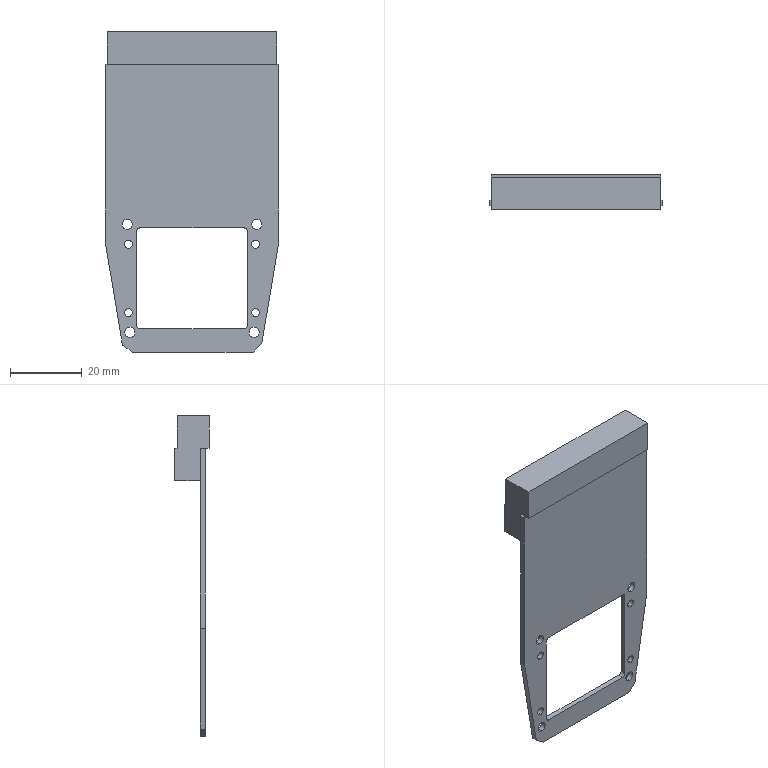Part | SolidWorks | features ICE 5, HoleWzd 2, LPattern 2, Chamfer 1, Cut 1, Extrusion 1, Fillet 1 | 1 solid | 128 faces | box 48 x 9.5 x 89 mm | volume 10809 mm3 | plane 84 | cylinder 44 | commonest cylinder face diameters 3 x24 2.2 x8 2.8 x8 2 x4